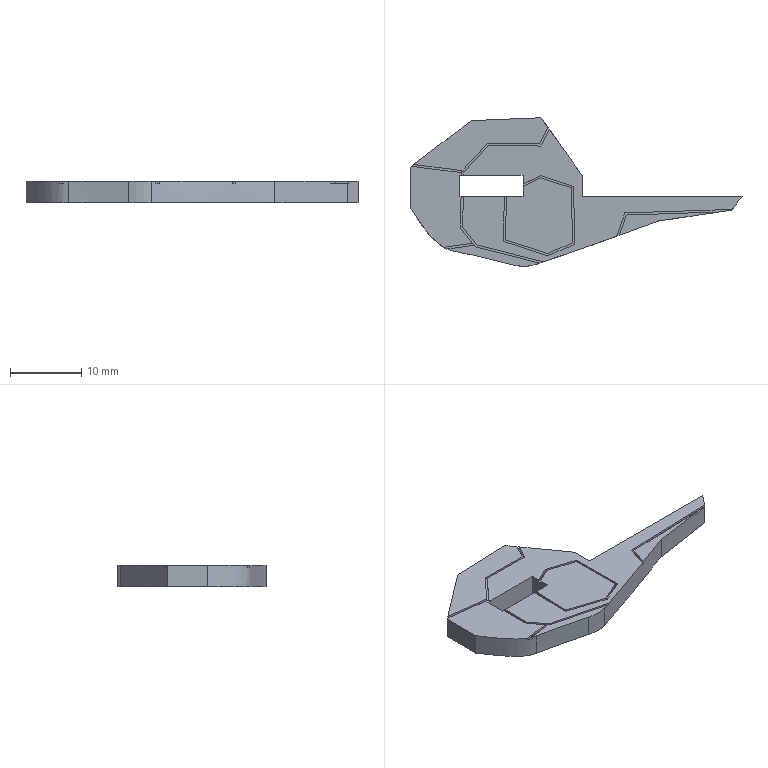Part | SolidWorks | features BaseBody 1 | 1 solid | 64 faces | box 46.751 x 20.92 x 3 mm | volume 1382 mm3 | plane 57 | spline 7